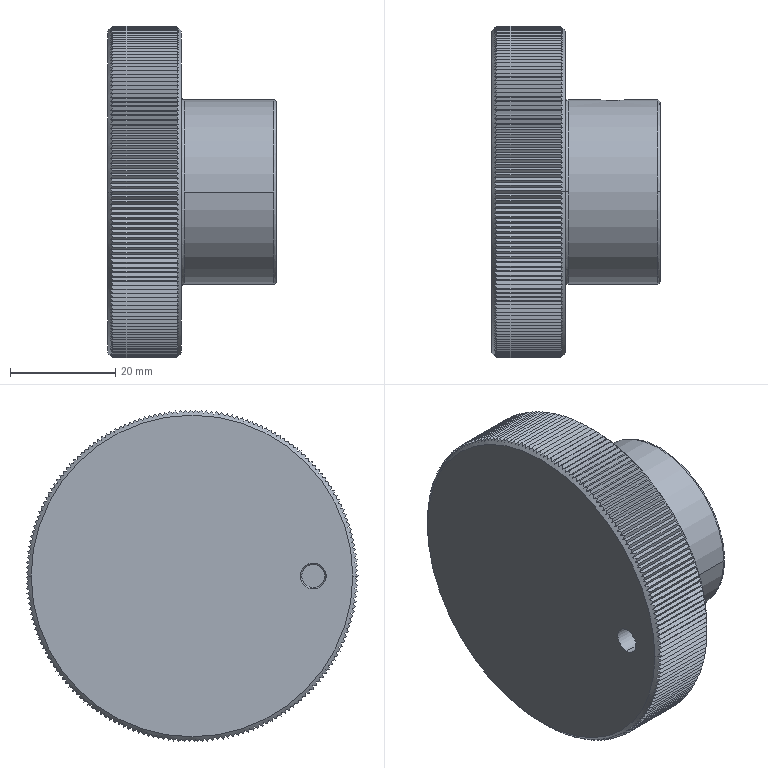Part | STEP file | 0232_Z_HOKW63_1 | 1 solid | 426 faces | box 32 x 62.998 x 62.995 mm | volume 57200 mm3 | plane 404 | cone 10 | cylinder 8 | spline 4 | commonest cylinder face diameters 4.134 x2 4.917 x2 12 x2 35 x2